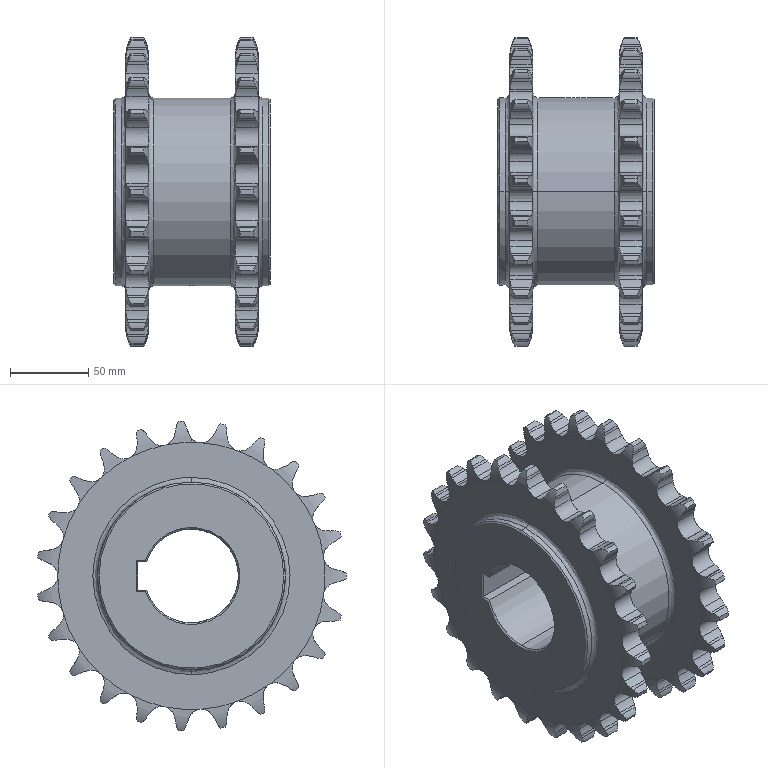Part | STEP file | 1 solid | 533 faces | box 100 x 197.271 x 197.721 mm | volume 1252435 mm3 | cylinder 313 | plane 107 | spline 104 | cone 9 | commonest cylinder face diameters 23.032 x98 41.467 x96 16.059 x60 198 x46 120 x6 10.2 x4